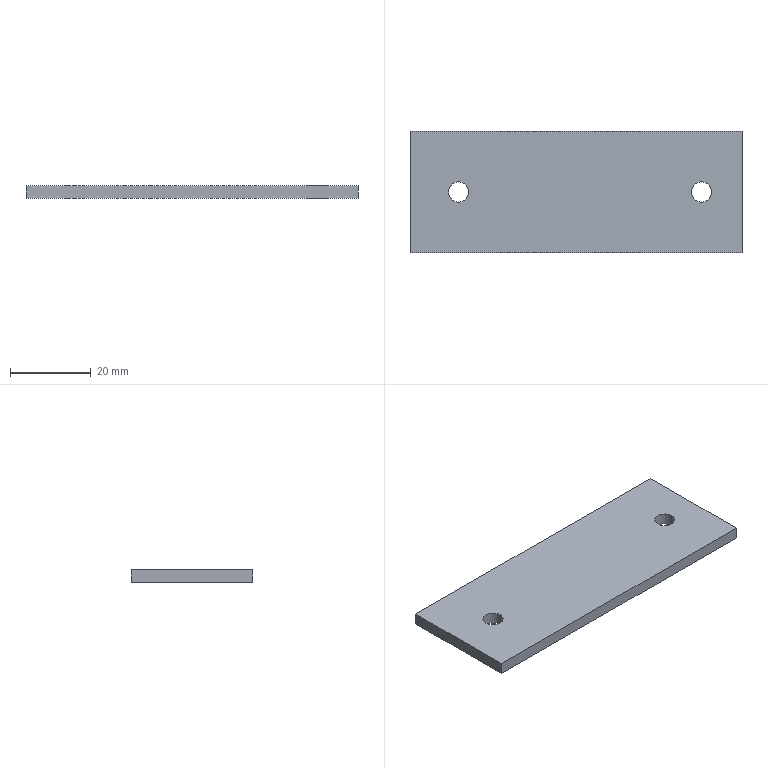Part | STEP file | Water guard fixing tab SGN-7-03 | 1 solid | 10 faces | box 82 x 30 x 3 mm | volume 7262 mm3 | plane 6 | cylinder 4 | commonest cylinder face diameters 5 x4
STEP:
#1=CARTESIAN_POINT('',(0.,0.,0.));
#2=DIRECTION('',(0.,0.,1.));
#3=DIRECTION('',(1.,0.,0.));
#4=AXIS2_PLACEMENT_3D('',#1,#2,#3);
#5=CARTESIAN_POINT('',(-26.5,0.,-3.));
#6=VERTEX_POINT('',#5);
#7=CARTESIAN_POINT('',(-26.5,0.,0.));
#8=VERTEX_POINT('',#7);
#9=CARTESIAN_POINT('',(-26.5,0.,0.));
#10=DIRECTION('',(0.,0.,1.));
#11=VECTOR('',#10,1.);
#12=LINE('',#9,#11);
#13=CARTESIAN_POINT('',(-29.,0.,0.));
#14=DIRECTION('',(0.,0.,1.));
#15=DIRECTION('',(1.,0.,0.));
#16=AXIS2_PLACEMENT_3D('',#13,#14,#15);
#17=CYLINDRICAL_SURFACE('',#16,2.5);
#18=CARTESIAN_POINT('',(6.283,0.));
#19=DIRECTION('',(0.,1.));
#20=VECTOR('',#19,1.);
#21=LINE('',#18,#20);
#22=(GEOMETRIC_REPRESENTATION_CONTEXT(2)PARAMETRIC_REPRESENTATION_CONTEXT()REPRESENTATION_CONTEXT('',''));
#23=DEFINITIONAL_REPRESENTATION('',(#21),#22);
#24=PCURVE('',#17,#23);
#25=CARTESIAN_POINT('',(-29.,0.,0.));
#26=DIRECTION('',(0.,0.,1.));
#27=DIRECTION('',(1.,0.,0.));
#28=AXIS2_PLACEMENT_3D('',#25,#26,#27);
#29=CYLINDRICAL_SURFACE('',#28,2.5);
#30=CARTESIAN_POINT('',(0.,0.));
#31=DIRECTION('',(0.,1.));
#32=VECTOR('',#31,1.);
#33=LINE('',#30,#32);
#34=(GEOMETRIC_REPRESENTATION_CONTEXT(2)PARAMETRIC_REPRESENTATION_CONTEXT()REPRESENTATION_CONTEXT('',''));
#35=DEFINITIONAL_REPRESENTATION('',(#33),#34);
#36=PCURVE('',#29,#35);
#37=SURFACE_CURVE('',#12,(#24,#36),.PCURVE_S1.);
#38=EDGE_CURVE('',#6,#8,#37,.T.);
#39=ORIENTED_EDGE('',*,*,#38,.T.);
#40=CARTESIAN_POINT('',(-31.5,0.,0.));
#41=VERTEX_POINT('',#40);
#42=CARTESIAN_POINT('',(-29.,0.,0.));
#43=DIRECTION('',(0.,0.,1.));
#44=DIRECTION('',(1.,0.,0.));
#45=AXIS2_PLACEMENT_3D('',#42,#43,#44);
#46=CIRCLE('',#45,2.5);
#47=CARTESIAN_POINT('',(0.,0.));
#48=DIRECTION('',(1.,0.));
#49=VECTOR('',#48,1.);
#50=LINE('',#47,#49);
#51=(GEOMETRIC_REPRESENTATION_CONTEXT(2)PARAMETRIC_REPRESENTATION_CONTEXT()REPRESENTATION_CONTEXT('',''));
#52=DEFINITIONAL_REPRESENTATION('',(#50),#51);
#53=PCURVE('',#17,#52);
#54=CARTESIAN_POINT('',(0.,0.,0.));
#55=DIRECTION('',(0.,0.,-1.));
#56=DIRECTION('',(-1.,0.,0.));
#57=AXIS2_PLACEMENT_3D('',#54,#55,#56);
#58=PLANE('',#57);
#59=CARTESIAN_POINT('',(26.5,0.));
#60=CARTESIAN_POINT('',(26.5,4.33));
#61=CARTESIAN_POINT('',(30.25,2.165));
#62=CARTESIAN_POINT('',(34.,0.));
#63=CARTESIAN_POINT('',(30.25,-2.165));
#64=CARTESIAN_POINT('',(26.5,-4.33));
#65=CARTESIAN_POINT('',(26.5,0.));
#66=(BOUNDED_CURVE()B_SPLINE_CURVE(2,(#59,#60,#61,#62,#63,#64,#65),.UNSPECIFIED.,.T.,.F.)B_SPLINE_CURVE_WITH_KNOTS((1,2,2,2,2,1),(-2.094,0.,2.094,4.189,6.283,8.378),.UNSPECIFIED.)CURVE()GEOMETRIC_REPRESENTATION_ITEM()RATIONAL_B_SPLINE_CURVE((1.,0.5,1.,0.5,1.,0.5,1.))REPRESENTATION_ITEM(''));
#67=(GEOMETRIC_REPRESENTATION_CONTEXT(2)PARAMETRIC_REPRESENTATION_CONTEXT()REPRESENTATION_CONTEXT('',''));
#68=DEFINITIONAL_REPRESENTATION('',(#66),#67);
#69=PCURVE('',#58,#68);
#70=SURFACE_CURVE('',#46,(#53,#69),.PCURVE_S1.);
#71=EDGE_CURVE('',#41,#8,#70,.T.);
#72=ORIENTED_EDGE('',*,*,#71,.F.);
#73=CARTESIAN_POINT('',(-31.5,0.,-3.));
#74=VERTEX_POINT('',#73);
#75=CARTESIAN_POINT('',(-31.5,0.,0.));
#76=DIRECTION('',(0.,0.,1.));
#77=VECTOR('',#76,1.);
#78=LINE('',#75,#77);
#79=CARTESIAN_POINT('',(3.142,0.));
#80=DIRECTION('',(0.,1.));
#81=VECTOR('',#80,1.);
#82=LINE('',#79,#81);
#83=(GEOMETRIC_REPRESENTATION_CONTEXT(2)PARAMETRIC_REPRESENTATION_CONTEXT()REPRESENTATION_CONTEXT('',''));
#84=DEFINITIONAL_REPRESENTATION('',(#82),#83);
#85=PCURVE('',#17,#84);
#86=CARTESIAN_POINT('',(3.142,0.));
#87=DIRECTION('',(0.,1.));
#88=VECTOR('',#87,1.);
#89=LINE('',#86,#88);
#90=(GEOMETRIC_REPRESENTATION_CONTEXT(2)PARAMETRIC_REPRESENTATION_CONTEXT()REPRESENTATION_CONTEXT('',''));
#91=DEFINITIONAL_REPRESENTATION('',(#89),#90);
#92=PCURVE('',#29,#91);
#93=SURFACE_CURVE('',#78,(#85,#92),.PCURVE_S1.);
#94=EDGE_CURVE('',#74,#41,#93,.T.);
#95=ORIENTED_EDGE('',*,*,#94,.F.);
#96=CARTESIAN_POINT('',(-29.,0.,-3.));
#97=DIRECTION('',(0.,0.,-1.));
#98=DIRECTION('',(-1.,0.,0.));
#99=AXIS2_PLACEMENT_3D('',#96,#97,#98);
#100=CIRCLE('',#99,2.5);
#101=CARTESIAN_POINT('',(9.425,-3.));
#102=DIRECTION('',(-1.,0.));
#103=VECTOR('',#102,1.);
#104=LINE('',#101,#103);
#105=(GEOMETRIC_REPRESENTATION_CONTEXT(2)PARAMETRIC_REPRESENTATION_CONTEXT()REPRESENTATION_CONTEXT('',''));
#106=DEFINITIONAL_REPRESENTATION('',(#104),#105);
#107=PCURVE('',#17,#106);
#108=CARTESIAN_POINT('',(0.,0.,-3.));
#109=DIRECTION('',(0.,0.,-1.));
#110=DIRECTION('',(-1.,0.,0.));
#111=AXIS2_PLACEMENT_3D('',#108,#109,#110);
#112=PLANE('',#111);
#113=CARTESIAN_POINT('',(29.,0.));
#114=DIRECTION('',(1.,0.));
#115=AXIS2_PLACEMENT_2D('',#113,#114);
#116=CIRCLE('',#115,2.5);
#117=(GEOMETRIC_REPRESENTATION_CONTEXT(2)PARAMETRIC_REPRESENTATION_CONTEXT()REPRESENTATION_CONTEXT('',''));
#118=DEFINITIONAL_REPRESENTATION('',(#116),#117);
#119=PCURVE('',#112,#118);
#120=SURFACE_CURVE('',#100,(#107,#119),.PCURVE_S1.);
#121=EDGE_CURVE('',#6,#74,#120,.T.);
#122=ORIENTED_EDGE('',*,*,#121,.F.);
#123=EDGE_LOOP('',(#39,#72,#95,#122));
#124=FACE_BOUND('',#123,.F.);
#125=ADVANCED_FACE('',(#124),#17,.F.);
#126=CARTESIAN_POINT('',(33.5,0.,-3.));
#127=VERTEX_POINT('',#126);
#128=CARTESIAN_POINT('',(33.5,0.,0.));
#129=VERTEX_POINT('',#128);
#130=CARTESIAN_POINT('',(33.5,0.,0.));
#131=DIRECTION('',(0.,0.,1.));
#132=VECTOR('',#131,1.);
#133=LINE('',#130,#132);
#134=CARTESIAN_POINT('',(31.,0.,0.));
#135=DIRECTION('',(0.,0.,1.));
#136=DIRECTION('',(1.,0.,0.));
#137=AXIS2_PLACEMENT_3D('',#134,#135,#136);
#138=CYLINDRICAL_SURFACE('',#137,2.5);
#139=CARTESIAN_POINT('',(6.283,0.));
#140=DIRECTION('',(0.,1.));
#141=VECTOR('',#140,1.);
#142=LINE('',#139,#141);
#143=(GEOMETRIC_REPRESENTATION_CONTEXT(2)PARAMETRIC_REPRESENTATION_CONTEXT()REPRESENTATION_CONTEXT('',''));
#144=DEFINITIONAL_REPRESENTATION('',(#142),#143);
#145=PCURVE('',#138,#144);
#146=CARTESIAN_POINT('',(31.,0.,0.));
#147=DIRECTION('',(0.,0.,1.));
#148=DIRECTION('',(1.,0.,0.));
#149=AXIS2_PLACEMENT_3D('',#146,#147,#148);
#150=CYLINDRICAL_SURFACE('',#149,2.5);
#151=CARTESIAN_POINT('',(0.,0.));
#152=DIRECTION('',(0.,1.));
#153=VECTOR('',#152,1.);
#154=LINE('',#151,#153);
#155=(GEOMETRIC_REPRESENTATION_CONTEXT(2)PARAMETRIC_REPRESENTATION_CONTEXT()REPRESENTATION_CONTEXT('',''));
#156=DEFINITIONAL_REPRESENTATION('',(#154),#155);
#157=PCURVE('',#150,#156);
#158=SURFACE_CURVE('',#133,(#145,#157),.PCURVE_S1.);
#159=EDGE_CURVE('',#127,#129,#158,.T.);
#160=ORIENTED_EDGE('',*,*,#159,.T.);
#161=CARTESIAN_POINT('',(28.5,0.,0.));
#162=VERTEX_POINT('',#161);
#163=CARTESIAN_POINT('',(31.,0.,0.));
#164=DIRECTION('',(0.,0.,1.));
#165=DIRECTION('',(1.,0.,0.));
#166=AXIS2_PLACEMENT_3D('',#163,#164,#165);
#167=CIRCLE('',#166,2.5);
#168=CARTESIAN_POINT('',(0.,0.));
#169=DIRECTION('',(1.,0.));
#170=VECTOR('',#169,1.);
#171=LINE('',#168,#170);
#172=(GEOMETRIC_REPRESENTATION_CONTEXT(2)PARAMETRIC_REPRESENTATION_CONTEXT()REPRESENTATION_CONTEXT('',''));
#173=DEFINITIONAL_REPRESENTATION('',(#171),#172);
#174=PCURVE('',#138,#173);
#175=CARTESIAN_POINT('',(-33.5,0.));
#176=CARTESIAN_POINT('',(-33.5,4.33));
#177=CARTESIAN_POINT('',(-29.75,2.165));
#178=CARTESIAN_POINT('',(-26.,0.));
#179=CARTESIAN_POINT('',(-29.75,-2.165));
#180=CARTESIAN_POINT('',(-33.5,-4.33));
#181=CARTESIAN_POINT('',(-33.5,0.));
#182=(BOUNDED_CURVE()B_SPLINE_CURVE(2,(#175,#176,#177,#178,#179,#180,#181),.UNSPECIFIED.,.T.,.F.)B_SPLINE_CURVE_WITH_KNOTS((1,2,2,2,2,1),(-2.094,0.,2.094,4.189,6.283,8.378),.UNSPECIFIED.)CURVE()GEOMETRIC_REPRESENTATION_ITEM()RATIONAL_B_SPLINE_CURVE((1.,0.5,1.,0.5,1.,0.5,1.))REPRESENTATION_ITEM(''));
#183=(GEOMETRIC_REPRESENTATION_CONTEXT(2)PARAMETRIC_REPRESENTATION_CONTEXT()REPRESENTATION_CONTEXT('',''));
#184=DEFINITIONAL_REPRESENTATION('',(#182),#183);
#185=PCURVE('',#58,#184);
#186=SURFACE_CURVE('',#167,(#174,#185),.PCURVE_S1.);
#187=EDGE_CURVE('',#162,#129,#186,.T.);
#188=ORIENTED_EDGE('',*,*,#187,.F.);
#189=CARTESIAN_POINT('',(28.5,0.,-3.));
#190=VERTEX_POINT('',#189);
#191=CARTESIAN_POINT('',(28.5,0.,0.));
#192=DIRECTION('',(0.,0.,1.));
#193=VECTOR('',#192,1.);
#194=LINE('',#191,#193);
#195=CARTESIAN_POINT('',(3.142,0.));
#196=DIRECTION('',(0.,1.));
#197=VECTOR('',#196,1.);
#198=LINE('',#195,#197);
#199=(GEOMETRIC_REPRESENTATION_CONTEXT(2)PARAMETRIC_REPRESENTATION_CONTEXT()REPRESENTATION_CONTEXT('',''));
#200=DEFINITIONAL_REPRESENTATION('',(#198),#199);
#201=PCURVE('',#138,#200);
#202=CARTESIAN_POINT('',(3.142,0.));
#203=DIRECTION('',(0.,1.));
#204=VECTOR('',#203,1.);
#205=LINE('',#202,#204);
#206=(GEOMETRIC_REPRESENTATION_CONTEXT(2)PARAMETRIC_REPRESENTATION_CONTEXT()REPRESENTATION_CONTEXT('',''));
#207=DEFINITIONAL_REPRESENTATION('',(#205),#206);
#208=PCURVE('',#150,#207);
#209=SURFACE_CURVE('',#194,(#201,#208),.PCURVE_S1.);
#210=EDGE_CURVE('',#190,#162,#209,.T.);
#211=ORIENTED_EDGE('',*,*,#210,.F.);
#212=CARTESIAN_POINT('',(31.,0.,-3.));
#213=DIRECTION('',(0.,0.,-1.));
#214=DIRECTION('',(-1.,0.,0.));
#215=AXIS2_PLACEMENT_3D('',#212,#213,#214);
#216=CIRCLE('',#215,2.5);
#217=CARTESIAN_POINT('',(9.425,-3.));
#218=DIRECTION('',(-1.,0.));
#219=VECTOR('',#218,1.);
#220=LINE('',#217,#219);
#221=(GEOMETRIC_REPRESENTATION_CONTEXT(2)PARAMETRIC_REPRESENTATION_CONTEXT()REPRESENTATION_CONTEXT('',''));
#222=DEFINITIONAL_REPRESENTATION('',(#220),#221);
#223=PCURVE('',#138,#222);
#224=CARTESIAN_POINT('',(-31.,0.));
#225=DIRECTION('',(1.,0.));
#226=AXIS2_PLACEMENT_2D('',#224,#225);
#227=CIRCLE('',#226,2.5);
#228=(GEOMETRIC_REPRESENTATION_CONTEXT(2)PARAMETRIC_REPRESENTATION_CONTEXT()REPRESENTATION_CONTEXT('',''));
#229=DEFINITIONAL_REPRESENTATION('',(#227),#228);
#230=PCURVE('',#112,#229);
#231=SURFACE_CURVE('',#216,(#223,#230),.PCURVE_S1.);
#232=EDGE_CURVE('',#127,#190,#231,.T.);
#233=ORIENTED_EDGE('',*,*,#232,.F.);
#234=EDGE_LOOP('',(#160,#188,#211,#233));
#235=FACE_BOUND('',#234,.F.);
#236=ADVANCED_FACE('',(#235),#138,.F.);
#237=CARTESIAN_POINT('',(41.,-15.,0.));
#238=VERTEX_POINT('',#237);
#239=CARTESIAN_POINT('',(41.,15.,0.));
#240=VERTEX_POINT('',#239);
#241=CARTESIAN_POINT('',(41.,-15.,0.));
#242=DIRECTION('',(0.,1.,0.));
#243=VECTOR('',#242,1.);
#244=LINE('',#241,#243);
#245=CARTESIAN_POINT('',(41.,-15.,-3.));
#246=DIRECTION('',(1.,0.,0.));
#247=DIRECTION('',(0.,0.,-1.));
#248=AXIS2_PLACEMENT_3D('',#245,#246,#247);
#249=PLANE('',#248);
#250=CARTESIAN_POINT('',(-3.,0.));
#251=DIRECTION('',(0.,1.));
#252=VECTOR('',#251,1.);
#253=LINE('',#250,#252);
#254=(GEOMETRIC_REPRESENTATION_CONTEXT(2)PARAMETRIC_REPRESENTATION_CONTEXT()REPRESENTATION_CONTEXT('',''));
#255=DEFINITIONAL_REPRESENTATION('',(#253),#254);
#256=PCURVE('',#249,#255);
#257=CARTESIAN_POINT('',(-41.,-15.));
#258=DIRECTION('',(0.,1.));
#259=VECTOR('',#258,1.);
#260=LINE('',#257,#259);
#261=(GEOMETRIC_REPRESENTATION_CONTEXT(2)PARAMETRIC_REPRESENTATION_CONTEXT()REPRESENTATION_CONTEXT('',''));
#262=DEFINITIONAL_REPRESENTATION('',(#260),#261);
#263=PCURVE('',#58,#262);
#264=SURFACE_CURVE('',#244,(#256,#263),.PCURVE_S1.);
#265=EDGE_CURVE('',#238,#240,#264,.T.);
#266=ORIENTED_EDGE('',*,*,#265,.F.);
#267=CARTESIAN_POINT('',(41.,-15.,-3.));
#268=VERTEX_POINT('',#267);
#269=CARTESIAN_POINT('',(41.,-15.,-3.));
#270=DIRECTION('',(0.,0.,1.));
#271=VECTOR('',#270,1.);
#272=LINE('',#269,#271);
#273=CARTESIAN_POINT('',(0.,0.));
#274=DIRECTION('',(-1.,0.));
#275=VECTOR('',#274,1.);
#276=LINE('',#273,#275);
#277=(GEOMETRIC_REPRESENTATION_CONTEXT(2)PARAMETRIC_REPRESENTATION_CONTEXT()REPRESENTATION_CONTEXT('',''));
#278=DEFINITIONAL_REPRESENTATION('',(#276),#277);
#279=PCURVE('',#249,#278);
#280=CARTESIAN_POINT('',(-41.,-15.,-3.));
#281=DIRECTION('',(0.,-1.,0.));
#282=DIRECTION('',(0.,0.,-1.));
#283=AXIS2_PLACEMENT_3D('',#280,#281,#282);
#284=PLANE('',#283);
#285=CARTESIAN_POINT('',(0.,82.));
#286=DIRECTION('',(-1.,0.));
#287=VECTOR('',#286,1.);
#288=LINE('',#285,#287);
#289=(GEOMETRIC_REPRESENTATION_CONTEXT(2)PARAMETRIC_REPRESENTATION_CONTEXT()REPRESENTATION_CONTEXT('',''));
#290=DEFINITIONAL_REPRESENTATION('',(#288),#289);
#291=PCURVE('',#284,#290);
#292=SURFACE_CURVE('',#272,(#279,#291),.PCURVE_S1.);
#293=EDGE_CURVE('',#268,#238,#292,.T.);
#294=ORIENTED_EDGE('',*,*,#293,.F.);
#295=CARTESIAN_POINT('',(41.,15.,-3.));
#296=VERTEX_POINT('',#295);
#297=CARTESIAN_POINT('',(41.,-15.,-3.));
#298=DIRECTION('',(0.,1.,0.));
#299=VECTOR('',#298,1.);
#300=LINE('',#297,#299);
#301=CARTESIAN_POINT('',(0.,0.));
#302=DIRECTION('',(0.,1.));
#303=VECTOR('',#302,1.);
#304=LINE('',#301,#303);
#305=(GEOMETRIC_REPRESENTATION_CONTEXT(2)PARAMETRIC_REPRESENTATION_CONTEXT()REPRESENTATION_CONTEXT('',''));
#306=DEFINITIONAL_REPRESENTATION('',(#304),#305);
#307=PCURVE('',#249,#306);
#308=CARTESIAN_POINT('',(-41.,-15.));
#309=DIRECTION('',(0.,1.));
#310=VECTOR('',#309,1.);
#311=LINE('',#308,#310);
#312=(GEOMETRIC_REPRESENTATION_CONTEXT(2)PARAMETRIC_REPRESENTATION_CONTEXT()REPRESENTATION_CONTEXT('',''));
#313=DEFINITIONAL_REPRESENTATION('',(#311),#312);
#314=PCURVE('',#112,#313);
#315=SURFACE_CURVE('',#300,(#307,#314),.PCURVE_S1.);
#316=EDGE_CURVE('',#268,#296,#315,.T.);
#317=ORIENTED_EDGE('',*,*,#316,.T.);
#318=CARTESIAN_POINT('',(41.,15.,-3.));
#319=DIRECTION('',(0.,0.,1.));
#320=VECTOR('',#319,1.);
#321=LINE('',#318,#320);
#322=CARTESIAN_POINT('',(0.,30.));
#323=DIRECTION('',(-1.,0.));
#324=VECTOR('',#323,1.);
#325=LINE('',#322,#324);
#326=(GEOMETRIC_REPRESENTATION_CONTEXT(2)PARAMETRIC_REPRESENTATION_CONTEXT()REPRESENTATION_CONTEXT('',''));
#327=DEFINITIONAL_REPRESENTATION('',(#325),#326);
#328=PCURVE('',#249,#327);
#329=CARTESIAN_POINT('',(-41.,15.,-3.));
#330=DIRECTION('',(0.,1.,0.));
#331=DIRECTION('',(0.,0.,1.));
#332=AXIS2_PLACEMENT_3D('',#329,#330,#331);
#333=PLANE('',#332);
#334=CARTESIAN_POINT('',(0.,82.));
#335=DIRECTION('',(1.,0.));
#336=VECTOR('',#335,1.);
#337=LINE('',#334,#336);
#338=(GEOMETRIC_REPRESENTATION_CONTEXT(2)PARAMETRIC_REPRESENTATION_CONTEXT()REPRESENTATION_CONTEXT('',''));
#339=DEFINITIONAL_REPRESENTATION('',(#337),#338);
#340=PCURVE('',#333,#339);
#341=SURFACE_CURVE('',#321,(#328,#340),.PCURVE_S1.);
#342=EDGE_CURVE('',#296,#240,#341,.T.);
#343=ORIENTED_EDGE('',*,*,#342,.T.);
#344=EDGE_LOOP('',(#266,#294,#317,#343));
#345=FACE_BOUND('',#344,.T.);
#346=ADVANCED_FACE('',(#345),#249,.T.);
#347=CARTESIAN_POINT('',(-41.,-15.,0.));
#348=VERTEX_POINT('',#347);
#349=CARTESIAN_POINT('',(-41.,-15.,0.));
#350=DIRECTION('',(1.,0.,0.));
#351=VECTOR('',#350,1.);
#352=LINE('',#349,#351);
#353=CARTESIAN_POINT('',(-3.,0.));
#354=DIRECTION('',(0.,1.));
#355=VECTOR('',#354,1.);
#356=LINE('',#353,#355);
#357=(GEOMETRIC_REPRESENTATION_CONTEXT(2)PARAMETRIC_REPRESENTATION_CONTEXT()REPRESENTATION_CONTEXT('',''));
#358=DEFINITIONAL_REPRESENTATION('',(#356),#357);
#359=PCURVE('',#284,#358);
#360=CARTESIAN_POINT('',(41.,-15.));
#361=DIRECTION('',(-1.,0.));
#362=VECTOR('',#361,1.);
#363=LINE('',#360,#362);
#364=(GEOMETRIC_REPRESENTATION_CONTEXT(2)PARAMETRIC_REPRESENTATION_CONTEXT()REPRESENTATION_CONTEXT('',''));
#365=DEFINITIONAL_REPRESENTATION('',(#363),#364);
#366=PCURVE('',#58,#365);
#367=SURFACE_CURVE('',#352,(#359,#366),.PCURVE_S1.);
#368=EDGE_CURVE('',#348,#238,#367,.T.);
#369=ORIENTED_EDGE('',*,*,#368,.F.);
#370=CARTESIAN_POINT('',(-41.,-15.,-3.));
#371=VERTEX_POINT('',#370);
#372=CARTESIAN_POINT('',(-41.,-15.,-3.));
#373=DIRECTION('',(0.,0.,1.));
#374=VECTOR('',#373,1.);
#375=LINE('',#372,#374);
#376=CARTESIAN_POINT('',(0.,0.));
#377=DIRECTION('',(-1.,0.));
#378=VECTOR('',#377,1.);
#379=LINE('',#376,#378);
#380=(GEOMETRIC_REPRESENTATION_CONTEXT(2)PARAMETRIC_REPRESENTATION_CONTEXT()REPRESENTATION_CONTEXT('',''));
#381=DEFINITIONAL_REPRESENTATION('',(#379),#380);
#382=PCURVE('',#284,#381);
#383=CARTESIAN_POINT('',(-41.,-15.,-3.));
#384=DIRECTION('',(-1.,0.,0.));
#385=DIRECTION('',(0.,0.,1.));
#386=AXIS2_PLACEMENT_3D('',#383,#384,#385);
#387=PLANE('',#386);
#388=CARTESIAN_POINT('',(0.,0.));
#389=DIRECTION('',(1.,0.));
#390=VECTOR('',#389,1.);
#391=LINE('',#388,#390);
#392=(GEOMETRIC_REPRESENTATION_CONTEXT(2)PARAMETRIC_REPRESENTATION_CONTEXT()REPRESENTATION_CONTEXT('',''));
#393=DEFINITIONAL_REPRESENTATION('',(#391),#392);
#394=PCURVE('',#387,#393);
#395=SURFACE_CURVE('',#375,(#382,#394),.PCURVE_S1.);
#396=EDGE_CURVE('',#371,#348,#395,.T.);
#397=ORIENTED_EDGE('',*,*,#396,.F.);
#398=CARTESIAN_POINT('',(-41.,-15.,-3.));
#399=DIRECTION('',(1.,0.,0.));
#400=VECTOR('',#399,1.);
#401=LINE('',#398,#400);
#402=CARTESIAN_POINT('',(0.,0.));
#403=DIRECTION('',(0.,1.));
#404=VECTOR('',#403,1.);
#405=LINE('',#402,#404);
#406=(GEOMETRIC_REPRESENTATION_CONTEXT(2)PARAMETRIC_REPRESENTATION_CONTEXT()REPRESENTATION_CONTEXT('',''));
#407=DEFINITIONAL_REPRESENTATION('',(#405),#406);
#408=PCURVE('',#284,#407);
#409=CARTESIAN_POINT('',(41.,-15.));
#410=DIRECTION('',(-1.,0.));
#411=VECTOR('',#410,1.);
#412=LINE('',#409,#411);
#413=(GEOMETRIC_REPRESENTATION_CONTEXT(2)PARAMETRIC_REPRESENTATION_CONTEXT()REPRESENTATION_CONTEXT('',''));
#414=DEFINITIONAL_REPRESENTATION('',(#412),#413);
#415=PCURVE('',#112,#414);
#416=SURFACE_CURVE('',#401,(#408,#415),.PCURVE_S1.);
#417=EDGE_CURVE('',#371,#268,#416,.T.);
#418=ORIENTED_EDGE('',*,*,#417,.T.);
#419=ORIENTED_EDGE('',*,*,#293,.T.);
#420=EDGE_LOOP('',(#369,#397,#418,#419));
#421=FACE_BOUND('',#420,.T.);
#422=ADVANCED_FACE('',(#421),#284,.T.);
#423=CARTESIAN_POINT('',(-41.,15.,0.));
#424=VERTEX_POINT('',#423);
#425=CARTESIAN_POINT('',(-41.,-15.,0.));
#426=DIRECTION('',(0.,-1.,0.));
#427=VECTOR('',#426,1.);
#428=LINE('',#425,#427);
#429=CARTESIAN_POINT('',(3.,0.));
#430=DIRECTION('',(0.,-1.));
#431=VECTOR('',#430,1.);
#432=LINE('',#429,#431);
#433=(GEOMETRIC_REPRESENTATION_CONTEXT(2)PARAMETRIC_REPRESENTATION_CONTEXT()REPRESENTATION_CONTEXT('',''));
#434=DEFINITIONAL_REPRESENTATION('',(#432),#433);
#435=PCURVE('',#387,#434);
#436=CARTESIAN_POINT('',(41.,-15.));
#437=DIRECTION('',(0.,-1.));
#438=VECTOR('',#437,1.);
#439=LINE('',#436,#438);
#440=(GEOMETRIC_REPRESENTATION_CONTEXT(2)PARAMETRIC_REPRESENTATION_CONTEXT()REPRESENTATION_CONTEXT('',''));
#441=DEFINITIONAL_REPRESENTATION('',(#439),#440);
#442=PCURVE('',#58,#441);
#443=SURFACE_CURVE('',#428,(#435,#442),.PCURVE_S1.);
#444=EDGE_CURVE('',#424,#348,#443,.T.);
#445=ORIENTED_EDGE('',*,*,#444,.F.);
#446=CARTESIAN_POINT('',(-41.,15.,-3.));
#447=VERTEX_POINT('',#446);
#448=CARTESIAN_POINT('',(-41.,15.,-3.));
#449=DIRECTION('',(0.,0.,1.));
#450=VECTOR('',#449,1.);
#451=LINE('',#448,#450);
#452=CARTESIAN_POINT('',(0.,30.));
#453=DIRECTION('',(1.,0.));
#454=VECTOR('',#453,1.);
#455=LINE('',#452,#454);
#456=(GEOMETRIC_REPRESENTATION_CONTEXT(2)PARAMETRIC_REPRESENTATION_CONTEXT()REPRESENTATION_CONTEXT('',''));
#457=DEFINITIONAL_REPRESENTATION('',(#455),#456);
#458=PCURVE('',#387,#457);
#459=CARTESIAN_POINT('',(0.,0.));
#460=DIRECTION('',(1.,0.));
#461=VECTOR('',#460,1.);
#462=LINE('',#459,#461);
#463=(GEOMETRIC_REPRESENTATION_CONTEXT(2)PARAMETRIC_REPRESENTATION_CONTEXT()REPRESENTATION_CONTEXT('',''));
#464=DEFINITIONAL_REPRESENTATION('',(#462),#463);
#465=PCURVE('',#333,#464);
#466=SURFACE_CURVE('',#451,(#458,#465),.PCURVE_S1.);
#467=EDGE_CURVE('',#447,#424,#466,.T.);
#468=ORIENTED_EDGE('',*,*,#467,.F.);
#469=CARTESIAN_POINT('',(-41.,-15.,-3.));
#470=DIRECTION('',(0.,-1.,0.));
#471=VECTOR('',#470,1.);
#472=LINE('',#469,#471);
#473=CARTESIAN_POINT('',(0.,0.));
#474=DIRECTION('',(0.,-1.));
#475=VECTOR('',#474,1.);
#476=LINE('',#473,#475);
#477=(GEOMETRIC_REPRESENTATION_CONTEXT(2)PARAMETRIC_REPRESENTATION_CONTEXT()REPRESENTATION_CONTEXT('',''));
#478=DEFINITIONAL_REPRESENTATION('',(#476),#477);
#479=PCURVE('',#387,#478);
#480=CARTESIAN_POINT('',(41.,-15.));
#481=DIRECTION('',(0.,-1.));
#482=VECTOR('',#481,1.);
#483=LINE('',#480,#482);
#484=(GEOMETRIC_REPRESENTATION_CONTEXT(2)PARAMETRIC_REPRESENTATION_CONTEXT()REPRESENTATION_CONTEXT('',''));
#485=DEFINITIONAL_REPRESENTATION('',(#483),#484);
#486=PCURVE('',#112,#485);
#487=SURFACE_CURVE('',#472,(#479,#486),.PCURVE_S1.);
#488=EDGE_CURVE('',#447,#371,#487,.T.);
#489=ORIENTED_EDGE('',*,*,#488,.T.);
#490=ORIENTED_EDGE('',*,*,#396,.T.);
#491=EDGE_LOOP('',(#445,#468,#489,#490));
#492=FACE_BOUND('',#491,.T.);
#493=ADVANCED_FACE('',(#492),#387,.T.);
#494=CARTESIAN_POINT('',(-41.,15.,0.));
#495=DIRECTION('',(-1.,0.,0.));
#496=VECTOR('',#495,1.);
#497=LINE('',#494,#496);
#498=CARTESIAN_POINT('',(3.,0.));
#499=DIRECTION('',(0.,-1.));
#500=VECTOR('',#499,1.);
#501=LINE('',#498,#500);
#502=(GEOMETRIC_REPRESENTATION_CONTEXT(2)PARAMETRIC_REPRESENTATION_CONTEXT()REPRESENTATION_CONTEXT('',''));
#503=DEFINITIONAL_REPRESENTATION('',(#501),#502);
#504=PCURVE('',#333,#503);
#505=CARTESIAN_POINT('',(41.,15.));
#506=DIRECTION('',(1.,0.));
#507=VECTOR('',#506,1.);
#508=LINE('',#505,#507);
#509=(GEOMETRIC_REPRESENTATION_CONTEXT(2)PARAMETRIC_REPRESENTATION_CONTEXT()REPRESENTATION_CONTEXT('',''));
#510=DEFINITIONAL_REPRESENTATION('',(#508),#509);
#511=PCURVE('',#58,#510);
#512=SURFACE_CURVE('',#497,(#504,#511),.PCURVE_S1.);
#513=EDGE_CURVE('',#240,#424,#512,.T.);
#514=ORIENTED_EDGE('',*,*,#513,.F.);
#515=ORIENTED_EDGE('',*,*,#342,.F.);
#516=CARTESIAN_POINT('',(-41.,15.,-3.));
#517=DIRECTION('',(-1.,0.,0.));
#518=VECTOR('',#517,1.);
#519=LINE('',#516,#518);
#520=CARTESIAN_POINT('',(0.,0.));
#521=DIRECTION('',(0.,-1.));
#522=VECTOR('',#521,1.);
#523=LINE('',#520,#522);
#524=(GEOMETRIC_REPRESENTATION_CONTEXT(2)PARAMETRIC_REPRESENTATION_CONTEXT()REPRESENTATION_CONTEXT('',''));
#525=DEFINITIONAL_REPRESENTATION('',(#523),#524);
#526=PCURVE('',#333,#525);
#527=CARTESIAN_POINT('',(41.,15.));
#528=DIRECTION('',(1.,0.));
#529=VECTOR('',#528,1.);
#530=LINE('',#527,#529);
#531=(GEOMETRIC_REPRESENTATION_CONTEXT(2)PARAMETRIC_REPRESENTATION_CONTEXT()REPRESENTATION_CONTEXT('',''));
#532=DEFINITIONAL_REPRESENTATION('',(#530),#531);
#533=PCURVE('',#112,#532);
#534=SURFACE_CURVE('',#519,(#526,#533),.PCURVE_S1.);
#535=EDGE_CURVE('',#296,#447,#534,.T.);
#536=ORIENTED_EDGE('',*,*,#535,.T.);
#537=ORIENTED_EDGE('',*,*,#467,.T.);
#538=EDGE_LOOP('',(#514,#515,#536,#537));
#539=FACE_BOUND('',#538,.T.);
#540=ADVANCED_FACE('',(#539),#333,.T.);
#541=ORIENTED_EDGE('',*,*,#121,.F.);
#542=CARTESIAN_POINT('',(-29.,0.,-3.));
#543=DIRECTION('',(0.,0.,-1.));
#544=DIRECTION('',(-1.,0.,0.));
#545=AXIS2_PLACEMENT_3D('',#542,#543,#544);
#546=CIRCLE('',#545,2.5);
#547=CARTESIAN_POINT('',(29.,0.));
#548=DIRECTION('',(1.,0.));
#549=AXIS2_PLACEMENT_2D('',#547,#548);
#550=CIRCLE('',#549,2.5);
#551=(GEOMETRIC_REPRESENTATION_CONTEXT(2)PARAMETRIC_REPRESENTATION_CONTEXT()REPRESENTATION_CONTEXT('',''));
#552=DEFINITIONAL_REPRESENTATION('',(#550),#551);
#553=PCURVE('',#112,#552);
#554=CARTESIAN_POINT('',(3.142,-3.));
#555=DIRECTION('',(-1.,0.));
#556=VECTOR('',#555,1.);
#557=LINE('',#554,#556);
#558=(GEOMETRIC_REPRESENTATION_CONTEXT(2)PARAMETRIC_REPRESENTATION_CONTEXT()REPRESENTATION_CONTEXT('',''));
#559=DEFINITIONAL_REPRESENTATION('',(#557),#558);
#560=PCURVE('',#29,#559);
#561=SURFACE_CURVE('',#546,(#553,#560),.PCURVE_S1.);
#562=EDGE_CURVE('',#74,#6,#561,.T.);
#563=ORIENTED_EDGE('',*,*,#562,.F.);
#564=EDGE_LOOP('',(#541,#563));
#565=FACE_BOUND('',#564,.T.);
#566=ORIENTED_EDGE('',*,*,#232,.F.);
#567=CARTESIAN_POINT('',(31.,0.,-3.));
#568=DIRECTION('',(0.,0.,-1.));
#569=DIRECTION('',(-1.,0.,0.));
#570=AXIS2_PLACEMENT_3D('',#567,#568,#569);
#571=CIRCLE('',#570,2.5);
#572=CARTESIAN_POINT('',(-31.,0.));
#573=DIRECTION('',(1.,0.));
#574=AXIS2_PLACEMENT_2D('',#572,#573);
#575=CIRCLE('',#574,2.5);
#576=(GEOMETRIC_REPRESENTATION_CONTEXT(2)PARAMETRIC_REPRESENTATION_CONTEXT()REPRESENTATION_CONTEXT('',''));
#577=DEFINITIONAL_REPRESENTATION('',(#575),#576);
#578=PCURVE('',#112,#577);
#579=CARTESIAN_POINT('',(3.142,-3.));
#580=DIRECTION('',(-1.,0.));
#581=VECTOR('',#580,1.);
#582=LINE('',#579,#581);
#583=(GEOMETRIC_REPRESENTATION_CONTEXT(2)PARAMETRIC_REPRESENTATION_CONTEXT()REPRESENTATION_CONTEXT('',''));
#584=DEFINITIONAL_REPRESENTATION('',(#582),#583);
#585=PCURVE('',#150,#584);
#586=SURFACE_CURVE('',#571,(#578,#585),.PCURVE_S1.);
#587=EDGE_CURVE('',#190,#127,#586,.T.);
#588=ORIENTED_EDGE('',*,*,#587,.F.);
#589=EDGE_LOOP('',(#566,#588));
#590=FACE_BOUND('',#589,.T.);
#591=ORIENTED_EDGE('',*,*,#316,.F.);
#592=ORIENTED_EDGE('',*,*,#417,.F.);
#593=ORIENTED_EDGE('',*,*,#488,.F.);
#594=ORIENTED_EDGE('',*,*,#535,.F.);
#595=EDGE_LOOP('',(#591,#592,#593,#594));
#596=FACE_BOUND('',#595,.T.);
#597=ADVANCED_FACE('',(#565,#590,#596),#112,.T.);
#598=CARTESIAN_POINT('',(-29.,0.,0.));
#599=DIRECTION('',(0.,0.,1.));
#600=DIRECTION('',(1.,0.,0.));
#601=AXIS2_PLACEMENT_3D('',#598,#599,#600);
#602=CIRCLE('',#601,2.5);
#603=CARTESIAN_POINT('',(26.5,0.));
#604=CARTESIAN_POINT('',(26.5,4.33));
#605=CARTESIAN_POINT('',(30.25,2.165));
#606=CARTESIAN_POINT('',(34.,0.));
#607=CARTESIAN_POINT('',(30.25,-2.165));
#608=CARTESIAN_POINT('',(26.5,-4.33));
#609=CARTESIAN_POINT('',(26.5,0.));
#610=(BOUNDED_CURVE()B_SPLINE_CURVE(2,(#603,#604,#605,#606,#607,#608,#609),.UNSPECIFIED.,.T.,.F.)B_SPLINE_CURVE_WITH_KNOTS((1,2,2,2,2,1),(-2.094,0.,2.094,4.189,6.283,8.378),.UNSPECIFIED.)CURVE()GEOMETRIC_REPRESENTATION_ITEM()RATIONAL_B_SPLINE_CURVE((1.,0.5,1.,0.5,1.,0.5,1.))REPRESENTATION_ITEM(''));
#611=(GEOMETRIC_REPRESENTATION_CONTEXT(2)PARAMETRIC_REPRESENTATION_CONTEXT()REPRESENTATION_CONTEXT('',''));
#612=DEFINITIONAL_REPRESENTATION('',(#610),#611);
#613=PCURVE('',#58,#612);
#614=CARTESIAN_POINT('',(0.,0.));
#615=DIRECTION('',(1.,0.));
#616=VECTOR('',#615,1.);
#617=LINE('',#614,#616);
#618=(GEOMETRIC_REPRESENTATION_CONTEXT(2)PARAMETRIC_REPRESENTATION_CONTEXT()REPRESENTATION_CONTEXT('',''));
#619=DEFINITIONAL_REPRESENTATION('',(#617),#618);
#620=PCURVE('',#29,#619);
#621=SURFACE_CURVE('',#602,(#613,#620),.PCURVE_S1.);
#622=EDGE_CURVE('',#8,#41,#621,.T.);
#623=ORIENTED_EDGE('',*,*,#622,.F.);
#624=ORIENTED_EDGE('',*,*,#71,.F.);
#625=EDGE_LOOP('',(#623,#624));
#626=FACE_BOUND('',#625,.T.);
#627=CARTESIAN_POINT('',(31.,0.,0.));
#628=DIRECTION('',(0.,0.,1.));
#629=DIRECTION('',(1.,0.,0.));
#630=AXIS2_PLACEMENT_3D('',#627,#628,#629);
#631=CIRCLE('',#630,2.5);
#632=CARTESIAN_POINT('',(-33.5,0.));
#633=CARTESIAN_POINT('',(-33.5,4.33));
#634=CARTESIAN_POINT('',(-29.75,2.165));
#635=CARTESIAN_POINT('',(-26.,0.));
#636=CARTESIAN_POINT('',(-29.75,-2.165));
#637=CARTESIAN_POINT('',(-33.5,-4.33));
#638=CARTESIAN_POINT('',(-33.5,0.));
#639=(BOUNDED_CURVE()B_SPLINE_CURVE(2,(#632,#633,#634,#635,#636,#637,#638),.UNSPECIFIED.,.T.,.F.)B_SPLINE_CURVE_WITH_KNOTS((1,2,2,2,2,1),(-2.094,0.,2.094,4.189,6.283,8.378),.UNSPECIFIED.)CURVE()GEOMETRIC_REPRESENTATION_ITEM()RATIONAL_B_SPLINE_CURVE((1.,0.5,1.,0.5,1.,0.5,1.))REPRESENTATION_ITEM(''));
#640=(GEOMETRIC_REPRESENTATION_CONTEXT(2)PARAMETRIC_REPRESENTATION_CONTEXT()REPRESENTATION_CONTEXT('',''));
#641=DEFINITIONAL_REPRESENTATION('',(#639),#640);
#642=PCURVE('',#58,#641);
#643=CARTESIAN_POINT('',(0.,0.));
#644=DIRECTION('',(1.,0.));
#645=VECTOR('',#644,1.);
#646=LINE('',#643,#645);
#647=(GEOMETRIC_REPRESENTATION_CONTEXT(2)PARAMETRIC_REPRESENTATION_CONTEXT()REPRESENTATION_CONTEXT('',''));
#648=DEFINITIONAL_REPRESENTATION('',(#646),#647);
#649=PCURVE('',#150,#648);
#650=SURFACE_CURVE('',#631,(#642,#649),.PCURVE_S1.);
#651=EDGE_CURVE('',#129,#162,#650,.T.);
#652=ORIENTED_EDGE('',*,*,#651,.F.);
#653=ORIENTED_EDGE('',*,*,#187,.F.);
#654=EDGE_LOOP('',(#652,#653));
#655=FACE_BOUND('',#654,.T.);
#656=ORIENTED_EDGE('',*,*,#265,.T.);
#657=ORIENTED_EDGE('',*,*,#513,.T.);
#658=ORIENTED_EDGE('',*,*,#444,.T.);
#659=ORIENTED_EDGE('',*,*,#368,.T.);
#660=EDGE_LOOP('',(#656,#657,#658,#659));
#661=FACE_BOUND('',#660,.T.);
#662=ADVANCED_FACE('',(#626,#655,#661),#58,.F.);
#663=ORIENTED_EDGE('',*,*,#651,.F.);
#664=ORIENTED_EDGE('',*,*,#159,.F.);
#665=ORIENTED_EDGE('',*,*,#587,.F.);
#666=ORIENTED_EDGE('',*,*,#210,.T.);
#667=EDGE_LOOP('',(#663,#664,#665,#666));
#668=FACE_BOUND('',#667,.F.);
#669=ADVANCED_FACE('',(#668),#150,.F.);
#670=ORIENTED_EDGE('',*,*,#622,.F.);
#671=ORIENTED_EDGE('',*,*,#38,.F.);
#672=ORIENTED_EDGE('',*,*,#562,.F.);
#673=ORIENTED_EDGE('',*,*,#94,.T.);
#674=EDGE_LOOP('',(#670,#671,#672,#673));
#675=FACE_BOUND('',#674,.F.);
#676=ADVANCED_FACE('',(#675),#29,.F.);
#677=CLOSED_SHELL('',(#125,#236,#346,#422,#493,#540,#597,#662,#669,#676));
#678=MANIFOLD_SOLID_BREP('',#677);
#679=(LENGTH_UNIT()NAMED_UNIT(*)SI_UNIT(.MILLI.,.METRE.));
#680=UNCERTAINTY_MEASURE_WITH_UNIT(LENGTH_MEASURE(0.0000001),#679,'','');
#681=(NAMED_UNIT(*)PLANE_ANGLE_UNIT()SI_UNIT($,.RADIAN.));
#682=(NAMED_UNIT(*)SI_UNIT($,.STERADIAN.)SOLID_ANGLE_UNIT());
#683=(GEOMETRIC_REPRESENTATION_CONTEXT(3)GLOBAL_UNCERTAINTY_ASSIGNED_CONTEXT((#680))GLOBAL_UNIT_ASSIGNED_CONTEXT((#679,#681,#682))REPRESENTATION_CONTEXT('',''));
#684=ADVANCED_BREP_SHAPE_REPRESENTATION('',(#4,#678),#683);